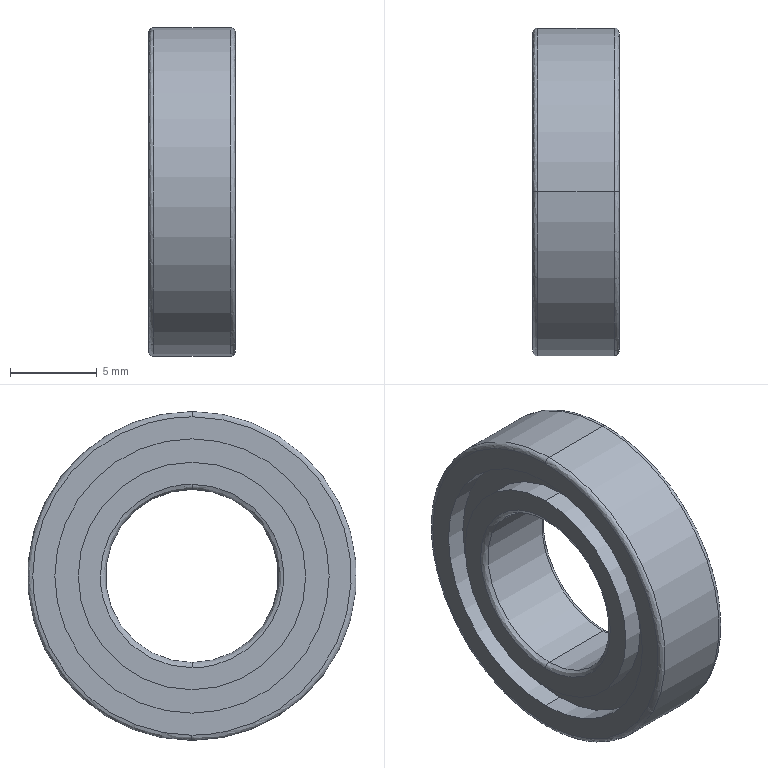Part | STEP file | B6800 | 1 solid | 26 faces | box 5 x 19 x 19 mm | volume 876.869 mm3 | cylinder 12 | spline 8 | plane 6 | commonest cylinder face diameters 13.15 x4 15.85 x4 10 x2 19 x2
STEP:
#1=CARTESIAN_POINT('',(0.,0.,9.2));
#2=VERTEX_POINT('',#1);
#3=CARTESIAN_POINT('',(0.,0.,-9.2));
#4=VERTEX_POINT('',#3);
#5=CARTESIAN_POINT('',(0.,0.,9.2));
#6=CARTESIAN_POINT('',(0.,-18.4,9.2));
#7=CARTESIAN_POINT('',(0.,-18.4,-9.2));
#8=CARTESIAN_POINT('',(0.,0.,-9.2));
#9=(BOUNDED_CURVE()B_SPLINE_CURVE(3,(#5,#6,#7,#8),.UNSPECIFIED.,.F.,.F.)B_SPLINE_CURVE_WITH_KNOTS((4,4),(0.,1.),.UNSPECIFIED.)CURVE()GEOMETRIC_REPRESENTATION_ITEM()RATIONAL_B_SPLINE_CURVE((1.,0.3333,0.3333,1.))REPRESENTATION_ITEM(''));
#10=EDGE_CURVE('',#2,#4,#9,.T.);
#11=ORIENTED_EDGE('',*,*,#10,.T.);
#12=CARTESIAN_POINT('',(0.3,0.,-9.5));
#13=VERTEX_POINT('',#12);
#14=CARTESIAN_POINT('',(0.3,0.,-9.2));
#15=DIRECTION('',(0.,-1.,0.));
#16=DIRECTION('',(0.,0.,-1.));
#17=AXIS2_PLACEMENT_3D('',#14,#15,#16);
#18=CIRCLE('',#17,0.3);
#19=EDGE_CURVE('',#4,#13,#18,.T.);
#20=ORIENTED_EDGE('',*,*,#19,.T.);
#21=CARTESIAN_POINT('',(0.3,0.,9.5));
#22=VERTEX_POINT('',#21);
#23=CARTESIAN_POINT('',(0.3,0.,0.));
#24=DIRECTION('',(1.,0.,0.));
#25=DIRECTION('',(0.,0.,-1.));
#26=AXIS2_PLACEMENT_3D('',#23,#24,#25);
#27=CIRCLE('',#26,9.5);
#28=EDGE_CURVE('',#22,#13,#27,.T.);
#29=ORIENTED_EDGE('',*,*,#28,.F.);
#30=CARTESIAN_POINT('',(0.3,0.,9.2));
#31=DIRECTION('',(0.,1.,0.));
#32=DIRECTION('',(0.,0.,1.));
#33=AXIS2_PLACEMENT_3D('',#30,#31,#32);
#34=CIRCLE('',#33,0.3);
#35=EDGE_CURVE('',#2,#22,#34,.T.);
#36=ORIENTED_EDGE('',*,*,#35,.F.);
#37=EDGE_LOOP('',(#11,#20,#29,#36));
#38=FACE_OUTER_BOUND('',#37,.T.);
#39=CARTESIAN_POINT('',(0.,0.,-9.2));
#40=CARTESIAN_POINT('',(0.,-18.4,-9.2));
#41=CARTESIAN_POINT('',(0.,-18.4,9.2));
#42=CARTESIAN_POINT('',(0.,0.,9.2));
#43=CARTESIAN_POINT('',(0.,0.,-9.376));
#44=CARTESIAN_POINT('',(0.,-18.751,-9.376));
#45=CARTESIAN_POINT('',(0.,-18.751,9.376));
#46=CARTESIAN_POINT('',(0.,0.,9.376));
#47=CARTESIAN_POINT('',(0.1243,0.,-9.5));
#48=CARTESIAN_POINT('',(0.1243,-19.,-9.5));
#49=CARTESIAN_POINT('',(0.1243,-19.,9.5));
#50=CARTESIAN_POINT('',(0.1243,0.,9.5));
#51=CARTESIAN_POINT('',(0.3,0.,-9.5));
#52=CARTESIAN_POINT('',(0.3,-19.,-9.5));
#53=CARTESIAN_POINT('',(0.3,-19.,9.5));
#54=CARTESIAN_POINT('',(0.3,0.,9.5));
#55=(BOUNDED_SURFACE()B_SPLINE_SURFACE(3,3,((#39,#40,#41,#42),(#43,#44,#45,#46),(#47,#48,#49,#50),(#51,#52,#53,#54)),.UNSPECIFIED.,.F.,.F.,.F.)B_SPLINE_SURFACE_WITH_KNOTS((4,4),(4,4),(0.,1.),(0.,1.),.UNSPECIFIED.)GEOMETRIC_REPRESENTATION_ITEM()RATIONAL_B_SPLINE_SURFACE(((1.,0.3333,0.3333,1.),(0.8047,0.2682,0.2682,0.8047),(0.8047,0.2682,0.2682,0.8047),(1.,0.3333,0.3333,1.)))REPRESENTATION_ITEM('')SURFACE());
#56=ADVANCED_FACE('',(#38),#55,.T.);
#57=CARTESIAN_POINT('',(4.7,0.,-9.5));
#58=VERTEX_POINT('',#57);
#59=CARTESIAN_POINT('',(4.7,0.,9.5));
#60=VERTEX_POINT('',#59);
#61=CARTESIAN_POINT('',(4.7,0.,0.));
#62=DIRECTION('',(-1.,0.,0.));
#63=DIRECTION('',(0.,0.,-1.));
#64=AXIS2_PLACEMENT_3D('',#61,#62,#63);
#65=CIRCLE('',#64,9.5);
#66=EDGE_CURVE('',#58,#60,#65,.T.);
#67=ORIENTED_EDGE('',*,*,#66,.F.);
#68=CARTESIAN_POINT('',(5.,0.,-9.2));
#69=VERTEX_POINT('',#68);
#70=CARTESIAN_POINT('',(4.7,0.,-9.2));
#71=DIRECTION('',(0.,-1.,0.));
#72=DIRECTION('',(0.,0.,-1.));
#73=AXIS2_PLACEMENT_3D('',#70,#71,#72);
#74=CIRCLE('',#73,0.3);
#75=EDGE_CURVE('',#58,#69,#74,.T.);
#76=ORIENTED_EDGE('',*,*,#75,.T.);
#77=CARTESIAN_POINT('',(5.,0.,9.2));
#78=VERTEX_POINT('',#77);
#79=CARTESIAN_POINT('',(5.,0.,-9.2));
#80=CARTESIAN_POINT('',(5.,-18.4,-9.2));
#81=CARTESIAN_POINT('',(5.,-18.4,9.2));
#82=CARTESIAN_POINT('',(5.,0.,9.2));
#83=(BOUNDED_CURVE()B_SPLINE_CURVE(3,(#79,#80,#81,#82),.UNSPECIFIED.,.F.,.F.)B_SPLINE_CURVE_WITH_KNOTS((4,4),(0.,1.),.UNSPECIFIED.)CURVE()GEOMETRIC_REPRESENTATION_ITEM()RATIONAL_B_SPLINE_CURVE((1.,0.3333,0.3333,1.))REPRESENTATION_ITEM(''));
#84=EDGE_CURVE('',#69,#78,#83,.T.);
#85=ORIENTED_EDGE('',*,*,#84,.T.);
#86=CARTESIAN_POINT('',(4.7,0.,9.2));
#87=DIRECTION('',(0.,1.,0.));
#88=DIRECTION('',(0.,0.,1.));
#89=AXIS2_PLACEMENT_3D('',#86,#87,#88);
#90=CIRCLE('',#89,0.3);
#91=EDGE_CURVE('',#60,#78,#90,.T.);
#92=ORIENTED_EDGE('',*,*,#91,.F.);
#93=EDGE_LOOP('',(#67,#76,#85,#92));
#94=FACE_OUTER_BOUND('',#93,.T.);
#95=CARTESIAN_POINT('',(4.7,0.,-9.5));
#96=CARTESIAN_POINT('',(4.7,-19.,-9.5));
#97=CARTESIAN_POINT('',(4.7,-19.,9.5));
#98=CARTESIAN_POINT('',(4.7,0.,9.5));
#99=CARTESIAN_POINT('',(4.876,0.,-9.5));
#100=CARTESIAN_POINT('',(4.876,-19.,-9.5));
#101=CARTESIAN_POINT('',(4.876,-19.,9.5));
#102=CARTESIAN_POINT('',(4.876,0.,9.5));
#103=CARTESIAN_POINT('',(5.,0.,-9.376));
#104=CARTESIAN_POINT('',(5.,-18.751,-9.376));
#105=CARTESIAN_POINT('',(5.,-18.751,9.376));
#106=CARTESIAN_POINT('',(5.,0.,9.376));
#107=CARTESIAN_POINT('',(5.,0.,-9.2));
#108=CARTESIAN_POINT('',(5.,-18.4,-9.2));
#109=CARTESIAN_POINT('',(5.,-18.4,9.2));
#110=CARTESIAN_POINT('',(5.,0.,9.2));
#111=(BOUNDED_SURFACE()B_SPLINE_SURFACE(3,3,((#95,#96,#97,#98),(#99,#100,#101,#102),(#103,#104,#105,#106),(#107,#108,#109,#110)),.UNSPECIFIED.,.F.,.F.,.F.)B_SPLINE_SURFACE_WITH_KNOTS((4,4),(4,4),(0.,1.),(0.,1.),.UNSPECIFIED.)GEOMETRIC_REPRESENTATION_ITEM()RATIONAL_B_SPLINE_SURFACE(((1.,0.3333,0.3333,1.),(0.8047,0.2682,0.2682,0.8047),(0.8047,0.2682,0.2682,0.8047),(1.,0.3333,0.3333,1.)))REPRESENTATION_ITEM('')SURFACE());
#112=ADVANCED_FACE('',(#94),#111,.T.);
#113=CARTESIAN_POINT('',(0.3,0.,5.));
#114=VERTEX_POINT('',#113);
#115=CARTESIAN_POINT('',(0.3,0.,-5.));
#116=VERTEX_POINT('',#115);
#117=CARTESIAN_POINT('',(0.3,0.,0.));
#118=DIRECTION('',(1.,0.,0.));
#119=DIRECTION('',(0.,0.,1.));
#120=AXIS2_PLACEMENT_3D('',#117,#118,#119);
#121=CIRCLE('',#120,5.);
#122=EDGE_CURVE('',#114,#116,#121,.T.);
#123=ORIENTED_EDGE('',*,*,#122,.T.);
#124=CARTESIAN_POINT('',(0.,0.,-5.3));
#125=VERTEX_POINT('',#124);
#126=CARTESIAN_POINT('',(0.3,0.,-5.3));
#127=DIRECTION('',(0.,-1.,0.));
#128=DIRECTION('',(0.,0.,-1.));
#129=AXIS2_PLACEMENT_3D('',#126,#127,#128);
#130=CIRCLE('',#129,0.3);
#131=EDGE_CURVE('',#116,#125,#130,.T.);
#132=ORIENTED_EDGE('',*,*,#131,.T.);
#133=CARTESIAN_POINT('',(0.,0.,5.3));
#134=VERTEX_POINT('',#133);
#135=CARTESIAN_POINT('',(0.,0.,5.3));
#136=CARTESIAN_POINT('',(0.,-0.3371,5.3));
#137=CARTESIAN_POINT('',(0.,-0.8337,5.253));
#138=CARTESIAN_POINT('',(0.,-1.398,5.118));
#139=CARTESIAN_POINT('',(0.,-1.676,5.03));
#140=CARTESIAN_POINT('',(0.,-1.814,4.98));
#141=CARTESIAN_POINT('',(0.,-1.872,4.958));
#142=CARTESIAN_POINT('',(0.,-1.912,4.943));
#143=CARTESIAN_POINT('',(0.,-1.93,4.936));
#144=CARTESIAN_POINT('',(0.,-2.117,4.862));
#145=CARTESIAN_POINT('',(0.,-2.361,4.751));
#146=CARTESIAN_POINT('',(0.,-2.595,4.622));
#147=CARTESIAN_POINT('',(0.,-2.749,4.532));
#148=CARTESIAN_POINT('',(0.,-2.824,4.486));
#149=CARTESIAN_POINT('',(0.,-3.206,4.236));
#150=CARTESIAN_POINT('',(0.,-3.489,4.006));
#151=CARTESIAN_POINT('',(0.,-3.877,3.618));
#152=CARTESIAN_POINT('',(0.,-4.06,3.416));
#153=CARTESIAN_POINT('',(0.,-4.227,3.199));
#154=CARTESIAN_POINT('',(0.,-4.334,3.052));
#155=CARTESIAN_POINT('',(0.,-4.387,2.975));
#156=CARTESIAN_POINT('',(0.,-4.534,2.75));
#157=CARTESIAN_POINT('',(0.,-4.669,2.519));
#158=CARTESIAN_POINT('',(0.,-4.805,2.239));
#159=CARTESIAN_POINT('',(0.,-4.859,2.116));
#160=CARTESIAN_POINT('',(0.,-4.894,2.034));
#161=CARTESIAN_POINT('',(0.,-4.912,1.991));
#162=CARTESIAN_POINT('',(0.,-4.991,1.791));
#163=CARTESIAN_POINT('',(0.,-5.074,1.548));
#164=CARTESIAN_POINT('',(0.,-5.15,1.258));
#165=CARTESIAN_POINT('',(0.,-5.182,1.112));
#166=CARTESIAN_POINT('',(0.,-5.195,1.049));
#167=CARTESIAN_POINT('',(0.,-5.204,1.007));
#168=CARTESIAN_POINT('',(0.,-5.208,0.9843));
#169=CARTESIAN_POINT('',(0.,-5.27,0.646));
#170=CARTESIAN_POINT('',(0.,-5.3,0.3238));
#171=CARTESIAN_POINT('',(0.,-5.3,-0.1619));
#172=CARTESIAN_POINT('',(0.,-5.289,-0.4039));
#173=CARTESIAN_POINT('',(0.,-5.257,-0.6847));
#174=CARTESIAN_POINT('',(0.,-5.236,-0.8247));
#175=CARTESIAN_POINT('',(0.,-5.226,-0.8846));
#176=CARTESIAN_POINT('',(0.,-5.219,-0.9245));
#177=CARTESIAN_POINT('',(0.,-5.215,-0.9433));
#178=CARTESIAN_POINT('',(0.,-5.18,-1.133));
#179=CARTESIAN_POINT('',(0.,-5.121,-1.383));
#180=CARTESIAN_POINT('',(0.,-5.032,-1.669));
#181=CARTESIAN_POINT('',(0.,-4.989,-1.79));
#182=CARTESIAN_POINT('',(0.,-4.959,-1.871));
#183=CARTESIAN_POINT('',(0.,-4.944,-1.909));
#184=CARTESIAN_POINT('',(0.,-4.862,-2.117));
#185=CARTESIAN_POINT('',(0.,-4.751,-2.361));
#186=CARTESIAN_POINT('',(0.,-4.622,-2.595));
#187=CARTESIAN_POINT('',(0.,-4.532,-2.749));
#188=CARTESIAN_POINT('',(0.,-4.486,-2.824));
#189=CARTESIAN_POINT('',(0.,-4.236,-3.206));
#190=CARTESIAN_POINT('',(0.,-4.006,-3.489));
#191=CARTESIAN_POINT('',(0.,-3.618,-3.877));
#192=CARTESIAN_POINT('',(0.,-3.416,-4.06));
#193=CARTESIAN_POINT('',(0.,-3.199,-4.227));
#194=CARTESIAN_POINT('',(0.,-3.052,-4.334));
#195=CARTESIAN_POINT('',(0.,-2.975,-4.387));
#196=CARTESIAN_POINT('',(0.,-2.75,-4.534));
#197=CARTESIAN_POINT('',(0.,-2.519,-4.669));
#198=CARTESIAN_POINT('',(0.,-2.239,-4.805));
#199=CARTESIAN_POINT('',(0.,-2.116,-4.859));
#200=CARTESIAN_POINT('',(0.,-2.034,-4.894));
#201=CARTESIAN_POINT('',(0.,-1.991,-4.912));
#202=CARTESIAN_POINT('',(0.,-1.791,-4.991));
#203=CARTESIAN_POINT('',(0.,-1.548,-5.074));
#204=CARTESIAN_POINT('',(0.,-1.258,-5.15));
#205=CARTESIAN_POINT('',(0.,-1.112,-5.182));
#206=CARTESIAN_POINT('',(0.,-1.049,-5.195));
#207=CARTESIAN_POINT('',(0.,-1.007,-5.204));
#208=CARTESIAN_POINT('',(0.,-0.9843,-5.208));
#209=CARTESIAN_POINT('',(0.,-0.6462,-5.27));
#210=CARTESIAN_POINT('',(0.,-0.3247,-5.3));
#211=CARTESIAN_POINT('',(0.,0.,-5.3));
#212=B_SPLINE_CURVE_WITH_KNOTS('',3,(#135,#136,#137,#138,#139,#140,#141,#142,#143,#144,#145,#146,#147,#148,#149,#150,#151,#152,#153,#154,#155,#156,#157,#158,#159,#160,#161,#162,#163,#164,#165,#166,#167,#168,#169,#170,#171,#172,#173,#174,#175,#176,#177,#178,#179,#180,#181,#182,#183,#184,#185,#186,#187,#188,#189,#190,#191,#192,#193,#194,#195,#196,#197,#198,#199,#200,#201,#202,#203,#204,#205,#206,#207,#208,#209,#210,#211),.UNSPECIFIED.,.F.,.F.,(4,1,1,1,1,2,2,1,2,2,2,1,2,2,1,1,2,2,1,1,1,2,2,2,1,1,1,2,2,1,1,2,2,1,2,2,2,1,2,2,1,1,2,2,1,1,1,2,2,4),(0.,0.0625,0.09375,0.1094,0.1172,0.1211,0.125,0.1563,0.1719,0.1875,0.25,0.2813,0.2969,0.3125,0.3438,0.3594,0.3672,0.375,0.4062,0.4219,0.4297,0.4336,0.4375,0.5,0.5312,0.5469,0.5547,0.5586,0.5625,0.5937,0.6094,0.6172,0.625,0.6562,0.6719,0.6875,0.75,0.7812,0.7969,0.8125,0.8437,0.8594,0.8672,0.875,0.9062,0.9219,0.9297,0.9336,0.9375,1.),.UNSPECIFIED.);
#213=EDGE_CURVE('',#134,#125,#212,.T.);
#214=ORIENTED_EDGE('',*,*,#213,.F.);
#215=CARTESIAN_POINT('',(0.3,0.,5.3));
#216=DIRECTION('',(0.,1.,0.));
#217=DIRECTION('',(0.,0.,1.));
#218=AXIS2_PLACEMENT_3D('',#215,#216,#217);
#219=CIRCLE('',#218,0.3);
#220=EDGE_CURVE('',#114,#134,#219,.T.);
#221=ORIENTED_EDGE('',*,*,#220,.F.);
#222=EDGE_LOOP('',(#123,#132,#214,#221));
#223=FACE_OUTER_BOUND('',#222,.T.);
#224=CARTESIAN_POINT('',(0.3,0.,-5.));
#225=CARTESIAN_POINT('',(0.3,-10.,-5.));
#226=CARTESIAN_POINT('',(0.3,-10.,5.));
#227=CARTESIAN_POINT('',(0.3,0.,5.));
#228=CARTESIAN_POINT('',(0.1243,0.,-5.));
#229=CARTESIAN_POINT('',(0.1243,-10.,-5.));
#230=CARTESIAN_POINT('',(0.1243,-10.,5.));
#231=CARTESIAN_POINT('',(0.1243,0.,5.));
#232=CARTESIAN_POINT('',(0.,0.,-5.124));
#233=CARTESIAN_POINT('',(0.,-10.249,-5.124));
#234=CARTESIAN_POINT('',(0.,-10.249,5.124));
#235=CARTESIAN_POINT('',(0.,0.,5.124));
#236=CARTESIAN_POINT('',(0.,0.,-5.3));
#237=CARTESIAN_POINT('',(0.,-10.6,-5.3));
#238=CARTESIAN_POINT('',(0.,-10.6,5.3));
#239=CARTESIAN_POINT('',(0.,0.,5.3));
#240=(BOUNDED_SURFACE()B_SPLINE_SURFACE(3,3,((#224,#225,#226,#227),(#228,#229,#230,#231),(#232,#233,#234,#235),(#236,#237,#238,#239)),.UNSPECIFIED.,.F.,.F.,.F.)B_SPLINE_SURFACE_WITH_KNOTS((4,4),(4,4),(0.,1.),(0.,1.),.UNSPECIFIED.)GEOMETRIC_REPRESENTATION_ITEM()RATIONAL_B_SPLINE_SURFACE(((1.,0.3333,0.3333,1.),(0.8047,0.2682,0.2682,0.8047),(0.8047,0.2682,0.2682,0.8047),(1.,0.3333,0.3333,1.)))REPRESENTATION_ITEM('')SURFACE());
#241=ADVANCED_FACE('',(#223),#240,.T.);
#242=CARTESIAN_POINT('',(5.,0.,-5.3));
#243=VERTEX_POINT('',#242);
#244=CARTESIAN_POINT('',(5.,0.,5.3));
#245=VERTEX_POINT('',#244);
#246=CARTESIAN_POINT('',(5.,0.,-5.3));
#247=CARTESIAN_POINT('',(5.,-0.3371,-5.3));
#248=CARTESIAN_POINT('',(5.,-0.8337,-5.253));
#249=CARTESIAN_POINT('',(5.,-1.398,-5.118));
#250=CARTESIAN_POINT('',(5.,-1.676,-5.03));
#251=CARTESIAN_POINT('',(5.,-1.814,-4.98));
#252=CARTESIAN_POINT('',(5.,-1.872,-4.958));
#253=CARTESIAN_POINT('',(5.,-1.912,-4.943));
#254=CARTESIAN_POINT('',(5.,-1.93,-4.936));
#255=CARTESIAN_POINT('',(5.,-2.117,-4.862));
#256=CARTESIAN_POINT('',(5.,-2.361,-4.751));
#257=CARTESIAN_POINT('',(5.,-2.595,-4.622));
#258=CARTESIAN_POINT('',(5.,-2.749,-4.532));
#259=CARTESIAN_POINT('',(5.,-2.824,-4.486));
#260=CARTESIAN_POINT('',(5.,-3.206,-4.236));
#261=CARTESIAN_POINT('',(5.,-3.489,-4.006));
#262=CARTESIAN_POINT('',(5.,-3.877,-3.618));
#263=CARTESIAN_POINT('',(5.,-4.06,-3.416));
#264=CARTESIAN_POINT('',(5.,-4.227,-3.199));
#265=CARTESIAN_POINT('',(5.,-4.334,-3.052));
#266=CARTESIAN_POINT('',(5.,-4.387,-2.975));
#267=CARTESIAN_POINT('',(5.,-4.534,-2.75));
#268=CARTESIAN_POINT('',(5.,-4.669,-2.519));
#269=CARTESIAN_POINT('',(5.,-4.805,-2.239));
#270=CARTESIAN_POINT('',(5.,-4.859,-2.116));
#271=CARTESIAN_POINT('',(5.,-4.894,-2.034));
#272=CARTESIAN_POINT('',(5.,-4.912,-1.991));
#273=CARTESIAN_POINT('',(5.,-4.991,-1.791));
#274=CARTESIAN_POINT('',(5.,-5.074,-1.548));
#275=CARTESIAN_POINT('',(5.,-5.15,-1.258));
#276=CARTESIAN_POINT('',(5.,-5.182,-1.112));
#277=CARTESIAN_POINT('',(5.,-5.195,-1.049));
#278=CARTESIAN_POINT('',(5.,-5.204,-1.007));
#279=CARTESIAN_POINT('',(5.,-5.208,-0.9843));
#280=CARTESIAN_POINT('',(5.,-5.27,-0.646));
#281=CARTESIAN_POINT('',(5.,-5.3,-0.3238));
#282=CARTESIAN_POINT('',(5.,-5.3,0.1619));
#283=CARTESIAN_POINT('',(5.,-5.289,0.4039));
#284=CARTESIAN_POINT('',(5.,-5.257,0.6847));
#285=CARTESIAN_POINT('',(5.,-5.236,0.8247));
#286=CARTESIAN_POINT('',(5.,-5.226,0.8846));
#287=CARTESIAN_POINT('',(5.,-5.219,0.9245));
#288=CARTESIAN_POINT('',(5.,-5.215,0.9433));
#289=CARTESIAN_POINT('',(5.,-5.18,1.133));
#290=CARTESIAN_POINT('',(5.,-5.121,1.383));
#291=CARTESIAN_POINT('',(5.,-5.032,1.669));
#292=CARTESIAN_POINT('',(5.,-4.989,1.79));
#293=CARTESIAN_POINT('',(5.,-4.959,1.871));
#294=CARTESIAN_POINT('',(5.,-4.944,1.909));
#295=CARTESIAN_POINT('',(5.,-4.862,2.117));
#296=CARTESIAN_POINT('',(5.,-4.751,2.361));
#297=CARTESIAN_POINT('',(5.,-4.622,2.595));
#298=CARTESIAN_POINT('',(5.,-4.532,2.749));
#299=CARTESIAN_POINT('',(5.,-4.486,2.824));
#300=CARTESIAN_POINT('',(5.,-4.236,3.206));
#301=CARTESIAN_POINT('',(5.,-4.006,3.489));
#302=CARTESIAN_POINT('',(5.,-3.618,3.877));
#303=CARTESIAN_POINT('',(5.,-3.416,4.06));
#304=CARTESIAN_POINT('',(5.,-3.199,4.227));
#305=CARTESIAN_POINT('',(5.,-3.052,4.334));
#306=CARTESIAN_POINT('',(5.,-2.975,4.387));
#307=CARTESIAN_POINT('',(5.,-2.75,4.534));
#308=CARTESIAN_POINT('',(5.,-2.519,4.669));
#309=CARTESIAN_POINT('',(5.,-2.239,4.805));
#310=CARTESIAN_POINT('',(5.,-2.116,4.859));
#311=CARTESIAN_POINT('',(5.,-2.034,4.894));
#312=CARTESIAN_POINT('',(5.,-1.991,4.912));
#313=CARTESIAN_POINT('',(5.,-1.791,4.991));
#314=CARTESIAN_POINT('',(5.,-1.548,5.074));
#315=CARTESIAN_POINT('',(5.,-1.258,5.15));
#316=CARTESIAN_POINT('',(5.,-1.112,5.182));
#317=CARTESIAN_POINT('',(5.,-1.049,5.195));
#318=CARTESIAN_POINT('',(5.,-1.007,5.204));
#319=CARTESIAN_POINT('',(5.,-0.9843,5.208));
#320=CARTESIAN_POINT('',(5.,-0.6462,5.27));
#321=CARTESIAN_POINT('',(5.,-0.3247,5.3));
#322=CARTESIAN_POINT('',(5.,0.,5.3));
#323=B_SPLINE_CURVE_WITH_KNOTS('',3,(#246,#247,#248,#249,#250,#251,#252,#253,#254,#255,#256,#257,#258,#259,#260,#261,#262,#263,#264,#265,#266,#267,#268,#269,#270,#271,#272,#273,#274,#275,#276,#277,#278,#279,#280,#281,#282,#283,#284,#285,#286,#287,#288,#289,#290,#291,#292,#293,#294,#295,#296,#297,#298,#299,#300,#301,#302,#303,#304,#305,#306,#307,#308,#309,#310,#311,#312,#313,#314,#315,#316,#317,#318,#319,#320,#321,#322),.UNSPECIFIED.,.F.,.F.,(4,1,1,1,1,2,2,1,2,2,2,1,2,2,1,1,2,2,1,1,1,2,2,2,1,1,1,2,2,1,1,2,2,1,2,2,2,1,2,2,1,1,2,2,1,1,1,2,2,4),(0.,0.0625,0.09375,0.1094,0.1172,0.1211,0.125,0.1563,0.1719,0.1875,0.25,0.2813,0.2969,0.3125,0.3438,0.3594,0.3672,0.375,0.4063,0.4219,0.4297,0.4336,0.4375,0.5,0.5312,0.5469,0.5547,0.5586,0.5625,0.5937,0.6094,0.6172,0.625,0.6562,0.6719,0.6875,0.75,0.7812,0.7969,0.8125,0.8437,0.8594,0.8672,0.875,0.9062,0.9219,0.9297,0.9336,0.9375,1.),.UNSPECIFIED.);
#324=EDGE_CURVE('',#243,#245,#323,.T.);
#325=ORIENTED_EDGE('',*,*,#324,.F.);
#326=CARTESIAN_POINT('',(4.7,0.,-5.));
#327=VERTEX_POINT('',#326);
#328=CARTESIAN_POINT('',(4.7,0.,-5.3));
#329=DIRECTION('',(0.,-1.,0.));
#330=DIRECTION('',(0.,0.,-1.));
#331=AXIS2_PLACEMENT_3D('',#328,#329,#330);
#332=CIRCLE('',#331,0.3);
#333=EDGE_CURVE('',#243,#327,#332,.T.);
#334=ORIENTED_EDGE('',*,*,#333,.T.);
#335=CARTESIAN_POINT('',(4.7,0.,5.));
#336=VERTEX_POINT('',#335);
#337=CARTESIAN_POINT('',(4.7,0.,0.));
#338=DIRECTION('',(-1.,0.,0.));
#339=DIRECTION('',(0.,0.,1.));
#340=AXIS2_PLACEMENT_3D('',#337,#338,#339);
#341=CIRCLE('',#340,5.);
#342=EDGE_CURVE('',#327,#336,#341,.T.);
#343=ORIENTED_EDGE('',*,*,#342,.T.);
#344=CARTESIAN_POINT('',(4.7,0.,5.3));
#345=DIRECTION('',(0.,1.,0.));
#346=DIRECTION('',(0.,0.,1.));
#347=AXIS2_PLACEMENT_3D('',#344,#345,#346);
#348=CIRCLE('',#347,0.3);
#349=EDGE_CURVE('',#245,#336,#348,.T.);
#350=ORIENTED_EDGE('',*,*,#349,.F.);
#351=EDGE_LOOP('',(#325,#334,#343,#350));
#352=FACE_OUTER_BOUND('',#351,.T.);
#353=CARTESIAN_POINT('',(5.,0.,-5.3));
#354=CARTESIAN_POINT('',(5.,-10.6,-5.3));
#355=CARTESIAN_POINT('',(5.,-10.6,5.3));
#356=CARTESIAN_POINT('',(5.,0.,5.3));
#357=CARTESIAN_POINT('',(5.,0.,-5.124));
#358=CARTESIAN_POINT('',(5.,-10.249,-5.124));
#359=CARTESIAN_POINT('',(5.,-10.249,5.124));
#360=CARTESIAN_POINT('',(5.,0.,5.124));
#361=CARTESIAN_POINT('',(4.876,0.,-5.));
#362=CARTESIAN_POINT('',(4.876,-10.,-5.));
#363=CARTESIAN_POINT('',(4.876,-10.,5.));
#364=CARTESIAN_POINT('',(4.876,0.,5.));
#365=CARTESIAN_POINT('',(4.7,0.,-5.));
#366=CARTESIAN_POINT('',(4.7,-10.,-5.));
#367=CARTESIAN_POINT('',(4.7,-10.,5.));
#368=CARTESIAN_POINT('',(4.7,0.,5.));
#369=(BOUNDED_SURFACE()B_SPLINE_SURFACE(3,3,((#353,#354,#355,#356),(#357,#358,#359,#360),(#361,#362,#363,#364),(#365,#366,#367,#368)),.UNSPECIFIED.,.F.,.F.,.F.)B_SPLINE_SURFACE_WITH_KNOTS((4,4),(4,4),(0.,1.),(0.,1.),.UNSPECIFIED.)GEOMETRIC_REPRESENTATION_ITEM()RATIONAL_B_SPLINE_SURFACE(((1.,0.3333,0.3333,1.),(0.8047,0.2682,0.2682,0.8047),(0.8047,0.2682,0.2682,0.8047),(1.,0.3333,0.3333,1.)))REPRESENTATION_ITEM('')SURFACE());
#370=ADVANCED_FACE('',(#352),#369,.T.);
#371=CARTESIAN_POINT('',(0.3,0.,0.));
#372=DIRECTION('',(1.,0.,0.));
#373=DIRECTION('',(0.,0.,-1.));
#374=AXIS2_PLACEMENT_3D('',#371,#372,#373);
#375=CIRCLE('',#374,9.5);
#376=EDGE_CURVE('',#13,#22,#375,.T.);
#377=ORIENTED_EDGE('',*,*,#376,.T.);
#378=CARTESIAN_POINT('',(2.5,0.,9.5));
#379=DIRECTION('',(1.,0.,0.));
#380=VECTOR('',#379,1000.);
#381=LINE('',#378,#380);
#382=EDGE_CURVE('',#22,#60,#381,.T.);
#383=ORIENTED_EDGE('',*,*,#382,.T.);
#384=CARTESIAN_POINT('',(4.7,0.,0.));
#385=DIRECTION('',(-1.,0.,0.));
#386=DIRECTION('',(0.,0.,-1.));
#387=AXIS2_PLACEMENT_3D('',#384,#385,#386);
#388=CIRCLE('',#387,9.5);
#389=EDGE_CURVE('',#60,#58,#388,.T.);
#390=ORIENTED_EDGE('',*,*,#389,.T.);
#391=CARTESIAN_POINT('',(2.5,0.,-9.5));
#392=DIRECTION('',(1.,0.,0.));
#393=VECTOR('',#392,1000.);
#394=LINE('',#391,#393);
#395=EDGE_CURVE('',#13,#58,#394,.T.);
#396=ORIENTED_EDGE('',*,*,#395,.F.);
#397=EDGE_LOOP('',(#377,#383,#390,#396));
#398=FACE_OUTER_BOUND('',#397,.T.);
#399=CARTESIAN_POINT('',(2.5,0.,0.));
#400=DIRECTION('',(1.,0.,0.));
#401=DIRECTION('',(0.,0.,-1.));
#402=AXIS2_PLACEMENT_3D('',#399,#400,#401);
#403=CYLINDRICAL_SURFACE('',#402,9.5);
#404=ADVANCED_FACE('',(#398),#403,.T.);
#405=CARTESIAN_POINT('',(0.,0.,7.925));
#406=VERTEX_POINT('',#405);
#407=CARTESIAN_POINT('',(0.,0.,-7.925));
#408=VERTEX_POINT('',#407);
#409=CARTESIAN_POINT('',(0.,0.,0.));
#410=DIRECTION('',(1.,0.,0.));
#411=DIRECTION('',(0.,0.,-1.));
#412=AXIS2_PLACEMENT_3D('',#409,#410,#411);
#413=CIRCLE('',#412,7.925);
#414=EDGE_CURVE('',#406,#408,#413,.T.);
#415=ORIENTED_EDGE('',*,*,#414,.F.);
#416=CARTESIAN_POINT('',(1.175,0.,7.925));
#417=VERTEX_POINT('',#416);
#418=CARTESIAN_POINT('',(0.5875,0.,7.925));
#419=DIRECTION('',(1.,0.,0.));
#420=VECTOR('',#419,1000.);
#421=LINE('',#418,#420);
#422=EDGE_CURVE('',#406,#417,#421,.T.);
#423=ORIENTED_EDGE('',*,*,#422,.T.);
#424=CARTESIAN_POINT('',(1.175,0.,-7.925));
#425=VERTEX_POINT('',#424);
#426=CARTESIAN_POINT('',(1.175,0.,0.));
#427=DIRECTION('',(-1.,0.,0.));
#428=DIRECTION('',(0.,0.,-1.));
#429=AXIS2_PLACEMENT_3D('',#426,#427,#428);
#430=CIRCLE('',#429,7.925);
#431=EDGE_CURVE('',#425,#417,#430,.T.);
#432=ORIENTED_EDGE('',*,*,#431,.F.);
#433=CARTESIAN_POINT('',(0.5875,0.,-7.925));
#434=DIRECTION('',(1.,0.,0.));
#435=VECTOR('',#434,1000.);
#436=LINE('',#433,#435);
#437=EDGE_CURVE('',#408,#425,#436,.T.);
#438=ORIENTED_EDGE('',*,*,#437,.F.);
#439=EDGE_LOOP('',(#415,#423,#432,#438));
#440=FACE_OUTER_BOUND('',#439,.T.);
#441=CARTESIAN_POINT('',(0.5875,0.,0.));
#442=DIRECTION('',(1.,0.,0.));
#443=DIRECTION('',(0.,0.,-1.));
#444=AXIS2_PLACEMENT_3D('',#441,#442,#443);
#445=CYLINDRICAL_SURFACE('',#444,7.925);
#446=ADVANCED_FACE('',(#440),#445,.F.);
#447=CARTESIAN_POINT('',(3.825,0.,7.925));
#448=VERTEX_POINT('',#447);
#449=CARTESIAN_POINT('',(3.825,0.,-7.925));
#450=VERTEX_POINT('',#449);
#451=CARTESIAN_POINT('',(3.825,0.,0.));
#452=DIRECTION('',(1.,0.,0.));
#453=DIRECTION('',(0.,0.,-1.));
#454=AXIS2_PLACEMENT_3D('',#451,#452,#453);
#455=CIRCLE('',#454,7.925);
#456=EDGE_CURVE('',#448,#450,#455,.T.);
#457=ORIENTED_EDGE('',*,*,#456,.F.);
#458=CARTESIAN_POINT('',(5.,0.,7.925));
#459=VERTEX_POINT('',#458);
#460=CARTESIAN_POINT('',(4.412,0.,7.925));
#461=DIRECTION('',(1.,0.,0.));
#462=VECTOR('',#461,1000.);
#463=LINE('',#460,#462);
#464=EDGE_CURVE('',#448,#459,#463,.T.);
#465=ORIENTED_EDGE('',*,*,#464,.T.);
#466=CARTESIAN_POINT('',(5.,0.,-7.925));
#467=VERTEX_POINT('',#466);
#468=CARTESIAN_POINT('',(5.,0.,0.));
#469=DIRECTION('',(-1.,0.,0.));
#470=DIRECTION('',(0.,0.,-1.));
#471=AXIS2_PLACEMENT_3D('',#468,#469,#470);
#472=CIRCLE('',#471,7.925);
#473=EDGE_CURVE('',#467,#459,#472,.T.);
#474=ORIENTED_EDGE('',*,*,#473,.F.);
#475=CARTESIAN_POINT('',(4.412,0.,-7.925));
#476=DIRECTION('',(1.,0.,0.));
#477=VECTOR('',#476,1000.);
#478=LINE('',#475,#477);
#479=EDGE_CURVE('',#450,#467,#478,.T.);
#480=ORIENTED_EDGE('',*,*,#479,.F.);
#481=EDGE_LOOP('',(#457,#465,#474,#480));
#482=FACE_OUTER_BOUND('',#481,.T.);
#483=CARTESIAN_POINT('',(4.412,0.,0.));
#484=DIRECTION('',(1.,0.,0.));
#485=DIRECTION('',(0.,0.,-1.));
#486=AXIS2_PLACEMENT_3D('',#483,#484,#485);
#487=CYLINDRICAL_SURFACE('',#486,7.925);
#488=ADVANCED_FACE('',(#482),#487,.F.);
#489=CARTESIAN_POINT('',(0.,0.,-6.575));
#490=VERTEX_POINT('',#489);
#491=CARTESIAN_POINT('',(0.,0.,6.575));
#492=VERTEX_POINT('',#491);
#493=CARTESIAN_POINT('',(0.,0.,0.));
#494=DIRECTION('',(1.,0.,0.));
#495=DIRECTION('',(0.,0.,-1.));
#496=AXIS2_PLACEMENT_3D('',#493,#494,#495);
#497=CIRCLE('',#496,6.575);
#498=EDGE_CURVE('',#490,#492,#497,.T.);
#499=ORIENTED_EDGE('',*,*,#498,.T.);
#500=CARTESIAN_POINT('',(1.175,0.,6.575));
#501=VERTEX_POINT('',#500);
#502=CARTESIAN_POINT('',(0.5875,0.,6.575));
#503=DIRECTION('',(1.,0.,0.));
#504=VECTOR('',#503,1000.);
#505=LINE('',#502,#504);
#506=EDGE_CURVE('',#492,#501,#505,.T.);
#507=ORIENTED_EDGE('',*,*,#506,.T.);
#508=CARTESIAN_POINT('',(1.175,0.,-6.575));
#509=VERTEX_POINT('',#508);
#510=CARTESIAN_POINT('',(1.175,0.,0.));
#511=DIRECTION('',(1.,0.,0.));
#512=DIRECTION('',(0.,0.,-1.));
#513=AXIS2_PLACEMENT_3D('',#510,#511,#512);
#514=CIRCLE('',#513,6.575);
#515=EDGE_CURVE('',#509,#501,#514,.T.);
#516=ORIENTED_EDGE('',*,*,#515,.F.);
#517=CARTESIAN_POINT('',(0.5875,0.,-6.575));
#518=DIRECTION('',(1.,0.,0.));
#519=VECTOR('',#518,1000.);
#520=LINE('',#517,#519);
#521=EDGE_CURVE('',#490,#509,#520,.T.);
#522=ORIENTED_EDGE('',*,*,#521,.F.);
#523=EDGE_LOOP('',(#499,#507,#516,#522));
#524=FACE_OUTER_BOUND('',#523,.T.);
#525=CARTESIAN_POINT('',(0.5875,0.,0.));
#526=DIRECTION('',(1.,0.,0.));
#527=DIRECTION('',(0.,0.,-1.));
#528=AXIS2_PLACEMENT_3D('',#525,#526,#527);
#529=CYLINDRICAL_SURFACE('',#528,6.575);
#530=ADVANCED_FACE('',(#524),#529,.T.);
#531=CARTESIAN_POINT('',(3.825,0.,6.575));
#532=VERTEX_POINT('',#531);
#533=CARTESIAN_POINT('',(3.825,0.,-6.575));
#534=VERTEX_POINT('',#533);
#535=CARTESIAN_POINT('',(3.825,0.,0.));
#536=DIRECTION('',(-1.,0.,0.));
#537=DIRECTION('',(0.,0.,-1.));
#538=AXIS2_PLACEMENT_3D('',#535,#536,#537);
#539=CIRCLE('',#538,6.575);
#540=EDGE_CURVE('',#532,#534,#539,.T.);
#541=ORIENTED_EDGE('',*,*,#540,.F.);
#542=CARTESIAN_POINT('',(5.,0.,6.575));
#543=VERTEX_POINT('',#542);
#544=CARTESIAN_POINT('',(4.412,0.,6.575));
#545=DIRECTION('',(1.,0.,0.));
#546=VECTOR('',#545,1000.);
#547=LINE('',#544,#546);
#548=EDGE_CURVE('',#532,#543,#547,.T.);
#549=ORIENTED_EDGE('',*,*,#548,.T.);
#550=CARTESIAN_POINT('',(5.,0.,-6.575));
#551=VERTEX_POINT('',#550);
#552=CARTESIAN_POINT('',(5.,0.,0.));
#553=DIRECTION('',(-1.,0.,0.));
#554=DIRECTION('',(0.,0.,-1.));
#555=AXIS2_PLACEMENT_3D('',#552,#553,#554);
#556=CIRCLE('',#555,6.575);
#557=EDGE_CURVE('',#543,#551,#556,.T.);
#558=ORIENTED_EDGE('',*,*,#557,.T.);
#559=CARTESIAN_POINT('',(4.412,0.,-6.575));
#560=DIRECTION('',(1.,0.,0.));
#561=VECTOR('',#560,1000.);
#562=LINE('',#559,#561);
#563=EDGE_CURVE('',#534,#551,#562,.T.);
#564=ORIENTED_EDGE('',*,*,#563,.F.);
#565=EDGE_LOOP('',(#541,#549,#558,#564));
#566=FACE_OUTER_BOUND('',#565,.T.);
#567=CARTESIAN_POINT('',(4.412,0.,0.));
#568=DIRECTION('',(1.,0.,0.));
#569=DIRECTION('',(0.,0.,-1.));
#570=AXIS2_PLACEMENT_3D('',#567,#568,#569);
#571=CYLINDRICAL_SURFACE('',#570,6.575);
#572=ADVANCED_FACE('',(#566),#571,.T.);
#573=ORIENTED_EDGE('',*,*,#122,.F.);
#574=CARTESIAN_POINT('',(2.5,0.,5.));
#575=DIRECTION('',(1.,0.,0.));
#576=VECTOR('',#575,1000.);
#577=LINE('',#574,#576);
#578=EDGE_CURVE('',#114,#336,#577,.T.);
#579=ORIENTED_EDGE('',*,*,#578,.T.);
#580=ORIENTED_EDGE('',*,*,#342,.F.);
#581=CARTESIAN_POINT('',(2.5,0.,-5.));
#582=DIRECTION('',(1.,0.,0.));
#583=VECTOR('',#582,1000.);
#584=LINE('',#581,#583);
#585=EDGE_CURVE('',#116,#327,#584,.T.);
#586=ORIENTED_EDGE('',*,*,#585,.F.);
#587=EDGE_LOOP('',(#573,#579,#580,#586));
#588=FACE_OUTER_BOUND('',#587,.T.);
#589=CARTESIAN_POINT('',(2.5,0.,0.));
#590=DIRECTION('',(1.,0.,0.));
#591=DIRECTION('',(0.,0.,-1.));
#592=AXIS2_PLACEMENT_3D('',#589,#590,#591);
#593=CYLINDRICAL_SURFACE('',#592,5.);
#594=ADVANCED_FACE('',(#588),#593,.F.);
#595=ORIENTED_EDGE('',*,*,#382,.F.);
#596=ORIENTED_EDGE('',*,*,#28,.T.);
#597=ORIENTED_EDGE('',*,*,#395,.T.);
#598=ORIENTED_EDGE('',*,*,#66,.T.);
#599=EDGE_LOOP('',(#595,#596,#597,#598));
#600=FACE_OUTER_BOUND('',#599,.T.);
#601=CARTESIAN_POINT('',(2.5,0.,0.));
#602=DIRECTION('',(1.,0.,0.));
#603=DIRECTION('',(0.,0.,-1.));
#604=AXIS2_PLACEMENT_3D('',#601,#602,#603);
#605=CYLINDRICAL_SURFACE('',#604,9.5);
#606=ADVANCED_FACE('',(#600),#605,.T.);
#607=ORIENTED_EDGE('',*,*,#19,.F.);
#608=CARTESIAN_POINT('',(0.,9.2,0.));
#609=VERTEX_POINT('',#608);
#610=CARTESIAN_POINT('',(0.,0.,-9.2));
#611=CARTESIAN_POINT('',(0.,5.389,-9.2));
#612=CARTESIAN_POINT('',(0.,9.2,-5.389));
#613=CARTESIAN_POINT('',(0.,9.2,0.));
#614=(BOUNDED_CURVE()B_SPLINE_CURVE(3,(#610,#611,#612,#613),.UNSPECIFIED.,.F.,.F.)B_SPLINE_CURVE_WITH_KNOTS((4,4),(0.,1.),.UNSPECIFIED.)CURVE()GEOMETRIC_REPRESENTATION_ITEM()RATIONAL_B_SPLINE_CURVE((1.,0.8047,0.8047,1.))REPRESENTATION_ITEM(''));
#615=EDGE_CURVE('',#4,#609,#614,.T.);
#616=ORIENTED_EDGE('',*,*,#615,.T.);
#617=CARTESIAN_POINT('',(0.,9.2,0.));
#618=CARTESIAN_POINT('',(0.,9.2,5.389));
#619=CARTESIAN_POINT('',(0.,5.389,9.2));
#620=CARTESIAN_POINT('',(0.,0.,9.2));
#621=(BOUNDED_CURVE()B_SPLINE_CURVE(3,(#617,#618,#619,#620),.UNSPECIFIED.,.F.,.F.)B_SPLINE_CURVE_WITH_KNOTS((4,4),(0.,1.),.UNSPECIFIED.)CURVE()GEOMETRIC_REPRESENTATION_ITEM()RATIONAL_B_SPLINE_CURVE((1.,0.8047,0.8047,1.))REPRESENTATION_ITEM(''));
#622=EDGE_CURVE('',#609,#2,#621,.T.);
#623=ORIENTED_EDGE('',*,*,#622,.T.);
#624=ORIENTED_EDGE('',*,*,#35,.T.);
#625=ORIENTED_EDGE('',*,*,#376,.F.);
#626=EDGE_LOOP('',(#607,#616,#623,#624,#625));
#627=FACE_OUTER_BOUND('',#626,.T.);
#628=CARTESIAN_POINT('',(0.,0.,9.2));
#629=CARTESIAN_POINT('',(0.,18.4,9.2));
#630=CARTESIAN_POINT('',(0.,18.4,-9.2));
#631=CARTESIAN_POINT('',(0.,0.,-9.2));
#632=CARTESIAN_POINT('',(0.,0.,9.376));
#633=CARTESIAN_POINT('',(0.,18.751,9.376));
#634=CARTESIAN_POINT('',(0.,18.751,-9.376));
#635=CARTESIAN_POINT('',(0.,0.,-9.376));
#636=CARTESIAN_POINT('',(0.1243,0.,9.5));
#637=CARTESIAN_POINT('',(0.1243,19.,9.5));
#638=CARTESIAN_POINT('',(0.1243,19.,-9.5));
#639=CARTESIAN_POINT('',(0.1243,0.,-9.5));
#640=CARTESIAN_POINT('',(0.3,0.,9.5));
#641=CARTESIAN_POINT('',(0.3,19.,9.5));
#642=CARTESIAN_POINT('',(0.3,19.,-9.5));
#643=CARTESIAN_POINT('',(0.3,0.,-9.5));
#644=(BOUNDED_SURFACE()B_SPLINE_SURFACE(3,3,((#628,#629,#630,#631),(#632,#633,#634,#635),(#636,#637,#638,#639),(#640,#641,#642,#643)),.UNSPECIFIED.,.F.,.F.,.F.)B_SPLINE_SURFACE_WITH_KNOTS((4,4),(4,4),(0.,1.),(0.,1.),.UNSPECIFIED.)GEOMETRIC_REPRESENTATION_ITEM()RATIONAL_B_SPLINE_SURFACE(((1.,0.3333,0.3333,1.),(0.8047,0.2682,0.2682,0.8047),(0.8047,0.2682,0.2682,0.8047),(1.,0.3333,0.3333,1.)))REPRESENTATION_ITEM('')SURFACE());
#645=ADVANCED_FACE('',(#627),#644,.T.);
#646=ORIENTED_EDGE('',*,*,#75,.F.);
#647=ORIENTED_EDGE('',*,*,#389,.F.);
#648=ORIENTED_EDGE('',*,*,#91,.T.);
#649=CARTESIAN_POINT('',(5.,9.2,0.));
#650=VERTEX_POINT('',#649);
#651=CARTESIAN_POINT('',(5.,0.,9.2));
#652=CARTESIAN_POINT('',(5.,5.389,9.2));
#653=CARTESIAN_POINT('',(5.,9.2,5.389));
#654=CARTESIAN_POINT('',(5.,9.2,0.));
#655=(BOUNDED_CURVE()B_SPLINE_CURVE(3,(#651,#652,#653,#654),.UNSPECIFIED.,.F.,.T.)B_SPLINE_CURVE_WITH_KNOTS((4,4),(0.,1.),.UNSPECIFIED.)CURVE()GEOMETRIC_REPRESENTATION_ITEM()RATIONAL_B_SPLINE_CURVE((1.,0.8047,0.8047,1.))REPRESENTATION_ITEM(''));
#656=EDGE_CURVE('',#78,#650,#655,.T.);
#657=ORIENTED_EDGE('',*,*,#656,.T.);
#658=CARTESIAN_POINT('',(5.,9.2,0.));
#659=CARTESIAN_POINT('',(5.,9.2,-5.389));
#660=CARTESIAN_POINT('',(5.,5.389,-9.2));
#661=CARTESIAN_POINT('',(5.,0.,-9.2));
#662=(BOUNDED_CURVE()B_SPLINE_CURVE(3,(#658,#659,#660,#661),.UNSPECIFIED.,.F.,.F.)B_SPLINE_CURVE_WITH_KNOTS((4,4),(0.,1.),.UNSPECIFIED.)CURVE()GEOMETRIC_REPRESENTATION_ITEM()RATIONAL_B_SPLINE_CURVE((1.,0.8047,0.8047,1.))REPRESENTATION_ITEM(''));
#663=EDGE_CURVE('',#650,#69,#662,.T.);
#664=ORIENTED_EDGE('',*,*,#663,.T.);
#665=EDGE_LOOP('',(#646,#647,#648,#657,#664));
#666=FACE_OUTER_BOUND('',#665,.T.);
#667=CARTESIAN_POINT('',(4.7,0.,9.5));
#668=CARTESIAN_POINT('',(4.7,19.,9.5));
#669=CARTESIAN_POINT('',(4.7,19.,-9.5));
#670=CARTESIAN_POINT('',(4.7,0.,-9.5));
#671=CARTESIAN_POINT('',(4.876,0.,9.5));
#672=CARTESIAN_POINT('',(4.876,19.,9.5));
#673=CARTESIAN_POINT('',(4.876,19.,-9.5));
#674=CARTESIAN_POINT('',(4.876,0.,-9.5));
#675=CARTESIAN_POINT('',(5.,0.,9.376));
#676=CARTESIAN_POINT('',(5.,18.751,9.376));
#677=CARTESIAN_POINT('',(5.,18.751,-9.376));
#678=CARTESIAN_POINT('',(5.,0.,-9.376));
#679=CARTESIAN_POINT('',(5.,0.,9.2));
#680=CARTESIAN_POINT('',(5.,18.4,9.2));
#681=CARTESIAN_POINT('',(5.,18.4,-9.2));
#682=CARTESIAN_POINT('',(5.,0.,-9.2));
#683=(BOUNDED_SURFACE()B_SPLINE_SURFACE(3,3,((#667,#668,#669,#670),(#671,#672,#673,#674),(#675,#676,#677,#678),(#679,#680,#681,#682)),.UNSPECIFIED.,.F.,.F.,.F.)B_SPLINE_SURFACE_WITH_KNOTS((4,4),(4,4),(0.,1.),(0.,1.),.UNSPECIFIED.)GEOMETRIC_REPRESENTATION_ITEM()RATIONAL_B_SPLINE_SURFACE(((1.,0.3333,0.3333,1.),(0.8047,0.2682,0.2682,0.8047),(0.8047,0.2682,0.2682,0.8047),(1.,0.3333,0.3333,1.)))REPRESENTATION_ITEM('')SURFACE());
#684=ADVANCED_FACE('',(#666),#683,.T.);
#685=ORIENTED_EDGE('',*,*,#10,.F.);
#686=ORIENTED_EDGE('',*,*,#622,.F.);
#687=ORIENTED_EDGE('',*,*,#615,.F.);
#688=EDGE_LOOP('',(#685,#686,#687));
#689=FACE_OUTER_BOUND('',#688,.T.);
#690=CARTESIAN_POINT('',(0.,0.,0.));
#691=DIRECTION('',(1.,0.,0.));
#692=DIRECTION('',(0.,0.,-1.));
#693=AXIS2_PLACEMENT_3D('',#690,#691,#692);
#694=CIRCLE('',#693,7.925);
#695=EDGE_CURVE('',#408,#406,#694,.T.);
#696=ORIENTED_EDGE('',*,*,#695,.T.);
#697=ORIENTED_EDGE('',*,*,#414,.T.);
#698=EDGE_LOOP('',(#696,#697));
#699=FACE_BOUND('',#698,.T.);
#700=CARTESIAN_POINT('',(0.,8.562,0.));
#701=DIRECTION('',(-1.,0.,0.));
#702=DIRECTION('',(0.,0.,1.));
#703=AXIS2_PLACEMENT_3D('',#700,#701,#702);
#704=PLANE('',#703);
#705=ADVANCED_FACE('',(#689,#699),#704,.T.);
#706=ORIENTED_EDGE('',*,*,#473,.T.);
#707=CARTESIAN_POINT('',(5.,0.,0.));
#708=DIRECTION('',(-1.,0.,0.));
#709=DIRECTION('',(0.,0.,-1.));
#710=AXIS2_PLACEMENT_3D('',#707,#708,#709);
#711=CIRCLE('',#710,7.925);
#712=EDGE_CURVE('',#459,#467,#711,.T.);
#713=ORIENTED_EDGE('',*,*,#712,.T.);
#714=EDGE_LOOP('',(#706,#713));
#715=FACE_BOUND('',#714,.T.);
#716=ORIENTED_EDGE('',*,*,#656,.F.);
#717=ORIENTED_EDGE('',*,*,#84,.F.);
#718=ORIENTED_EDGE('',*,*,#663,.F.);
#719=EDGE_LOOP('',(#716,#717,#718));
#720=FACE_OUTER_BOUND('',#719,.T.);
#721=CARTESIAN_POINT('',(5.,8.562,0.));
#722=DIRECTION('',(1.,0.,0.));
#723=DIRECTION('',(0.,0.,-1.));
#724=AXIS2_PLACEMENT_3D('',#721,#722,#723);
#725=PLANE('',#724);
#726=ADVANCED_FACE('',(#715,#720),#725,.T.);
#727=ORIENTED_EDGE('',*,*,#422,.F.);
#728=ORIENTED_EDGE('',*,*,#695,.F.);
#729=ORIENTED_EDGE('',*,*,#437,.T.);
#730=CARTESIAN_POINT('',(1.175,0.,0.));
#731=DIRECTION('',(-1.,0.,0.));
#732=DIRECTION('',(0.,0.,-1.));
#733=AXIS2_PLACEMENT_3D('',#730,#731,#732);
#734=CIRCLE('',#733,7.925);
#735=EDGE_CURVE('',#417,#425,#734,.T.);
#736=ORIENTED_EDGE('',*,*,#735,.F.);
#737=EDGE_LOOP('',(#727,#728,#729,#736));
#738=FACE_OUTER_BOUND('',#737,.T.);
#739=CARTESIAN_POINT('',(0.5875,0.,0.));
#740=DIRECTION('',(1.,0.,0.));
#741=DIRECTION('',(0.,0.,-1.));
#742=AXIS2_PLACEMENT_3D('',#739,#740,#741);
#743=CYLINDRICAL_SURFACE('',#742,7.925);
#744=ADVANCED_FACE('',(#738),#743,.F.);
#745=ORIENTED_EDGE('',*,*,#464,.F.);
#746=CARTESIAN_POINT('',(3.825,0.,0.));
#747=DIRECTION('',(1.,0.,0.));
#748=DIRECTION('',(0.,0.,-1.));
#749=AXIS2_PLACEMENT_3D('',#746,#747,#748);
#750=CIRCLE('',#749,7.925);
#751=EDGE_CURVE('',#450,#448,#750,.T.);
#752=ORIENTED_EDGE('',*,*,#751,.F.);
#753=ORIENTED_EDGE('',*,*,#479,.T.);
#754=ORIENTED_EDGE('',*,*,#712,.F.);
#755=EDGE_LOOP('',(#745,#752,#753,#754));
#756=FACE_OUTER_BOUND('',#755,.T.);
#757=CARTESIAN_POINT('',(4.412,0.,0.));
#758=DIRECTION('',(1.,0.,0.));
#759=DIRECTION('',(0.,0.,-1.));
#760=AXIS2_PLACEMENT_3D('',#757,#758,#759);
#761=CYLINDRICAL_SURFACE('',#760,7.925);
#762=ADVANCED_FACE('',(#756),#761,.F.);
#763=ORIENTED_EDGE('',*,*,#431,.T.);
#764=ORIENTED_EDGE('',*,*,#735,.T.);
#765=EDGE_LOOP('',(#763,#764));
#766=FACE_OUTER_BOUND('',#765,.T.);
#767=ORIENTED_EDGE('',*,*,#515,.T.);
#768=CARTESIAN_POINT('',(1.175,0.,0.));
#769=DIRECTION('',(1.,0.,0.));
#770=DIRECTION('',(0.,0.,-1.));
#771=AXIS2_PLACEMENT_3D('',#768,#769,#770);
#772=CIRCLE('',#771,6.575);
#773=EDGE_CURVE('',#501,#509,#772,.T.);
#774=ORIENTED_EDGE('',*,*,#773,.T.);
#775=EDGE_LOOP('',(#767,#774));
#776=FACE_BOUND('',#775,.T.);
#777=CARTESIAN_POINT('',(1.175,7.25,0.));
#778=DIRECTION('',(-1.,0.,0.));
#779=DIRECTION('',(0.,0.,1.));
#780=AXIS2_PLACEMENT_3D('',#777,#778,#779);
#781=PLANE('',#780);
#782=ADVANCED_FACE('',(#766,#776),#781,.T.);
#783=CARTESIAN_POINT('',(3.825,0.,0.));
#784=DIRECTION('',(-1.,0.,0.));
#785=DIRECTION('',(0.,0.,-1.));
#786=AXIS2_PLACEMENT_3D('',#783,#784,#785);
#787=CIRCLE('',#786,6.575);
#788=EDGE_CURVE('',#534,#532,#787,.T.);
#789=ORIENTED_EDGE('',*,*,#788,.T.);
#790=ORIENTED_EDGE('',*,*,#540,.T.);
#791=EDGE_LOOP('',(#789,#790));
#792=FACE_BOUND('',#791,.T.);
#793=ORIENTED_EDGE('',*,*,#751,.T.);
#794=ORIENTED_EDGE('',*,*,#456,.T.);
#795=EDGE_LOOP('',(#793,#794));
#796=FACE_OUTER_BOUND('',#795,.T.);
#797=CARTESIAN_POINT('',(3.825,7.25,0.));
#798=DIRECTION('',(1.,0.,0.));
#799=DIRECTION('',(0.,0.,-1.));
#800=AXIS2_PLACEMENT_3D('',#797,#798,#799);
#801=PLANE('',#800);
#802=ADVANCED_FACE('',(#792,#796),#801,.T.);
#803=ORIENTED_EDGE('',*,*,#506,.F.);
#804=CARTESIAN_POINT('',(0.,0.,0.));
#805=DIRECTION('',(1.,0.,0.));
#806=DIRECTION('',(0.,0.,-1.));
#807=AXIS2_PLACEMENT_3D('',#804,#805,#806);
#808=CIRCLE('',#807,6.575);
#809=EDGE_CURVE('',#492,#490,#808,.T.);
#810=ORIENTED_EDGE('',*,*,#809,.T.);
#811=ORIENTED_EDGE('',*,*,#521,.T.);
#812=ORIENTED_EDGE('',*,*,#773,.F.);
#813=EDGE_LOOP('',(#803,#810,#811,#812));
#814=FACE_OUTER_BOUND('',#813,.T.);
#815=CARTESIAN_POINT('',(0.5875,0.,0.));
#816=DIRECTION('',(1.,0.,0.));
#817=DIRECTION('',(0.,0.,-1.));
#818=AXIS2_PLACEMENT_3D('',#815,#816,#817);
#819=CYLINDRICAL_SURFACE('',#818,6.575);
#820=ADVANCED_FACE('',(#814),#819,.T.);
#821=ORIENTED_EDGE('',*,*,#548,.F.);
#822=ORIENTED_EDGE('',*,*,#788,.F.);
#823=ORIENTED_EDGE('',*,*,#563,.T.);
#824=CARTESIAN_POINT('',(5.,0.,0.));
#825=DIRECTION('',(-1.,0.,0.));
#826=DIRECTION('',(0.,0.,-1.));
#827=AXIS2_PLACEMENT_3D('',#824,#825,#826);
#828=CIRCLE('',#827,6.575);
#829=EDGE_CURVE('',#551,#543,#828,.T.);
#830=ORIENTED_EDGE('',*,*,#829,.T.);
#831=EDGE_LOOP('',(#821,#822,#823,#830));
#832=FACE_OUTER_BOUND('',#831,.T.);
#833=CARTESIAN_POINT('',(4.412,0.,0.));
#834=DIRECTION('',(1.,0.,0.));
#835=DIRECTION('',(0.,0.,-1.));
#836=AXIS2_PLACEMENT_3D('',#833,#834,#835);
#837=CYLINDRICAL_SURFACE('',#836,6.575);
#838=ADVANCED_FACE('',(#832),#837,.T.);
#839=ORIENTED_EDGE('',*,*,#498,.F.);
#840=ORIENTED_EDGE('',*,*,#809,.F.);
#841=EDGE_LOOP('',(#839,#840));
#842=FACE_OUTER_BOUND('',#841,.T.);
#843=CARTESIAN_POINT('',(0.,5.3,0.));
#844=VERTEX_POINT('',#843);
#845=CARTESIAN_POINT('',(0.,5.3,0.));
#846=CARTESIAN_POINT('',(0.,5.3,0.3371));
#847=CARTESIAN_POINT('',(0.,5.253,0.8337));
#848=CARTESIAN_POINT('',(0.,5.118,1.398));
#849=CARTESIAN_POINT('',(0.,5.03,1.676));
#850=CARTESIAN_POINT('',(0.,4.98,1.814));
#851=CARTESIAN_POINT('',(0.,4.958,1.872));
#852=CARTESIAN_POINT('',(0.,4.943,1.912));
#853=CARTESIAN_POINT('',(0.,4.936,1.93));
#854=CARTESIAN_POINT('',(0.,4.862,2.117));
#855=CARTESIAN_POINT('',(0.,4.751,2.361));
#856=CARTESIAN_POINT('',(0.,4.622,2.595));
#857=CARTESIAN_POINT('',(0.,4.532,2.749));
#858=CARTESIAN_POINT('',(0.,4.486,2.824));
#859=CARTESIAN_POINT('',(0.,4.236,3.206));
#860=CARTESIAN_POINT('',(0.,4.006,3.489));
#861=CARTESIAN_POINT('',(0.,3.618,3.877));
#862=CARTESIAN_POINT('',(0.,3.416,4.06));
#863=CARTESIAN_POINT('',(0.,3.199,4.227));
#864=CARTESIAN_POINT('',(0.,3.052,4.334));
#865=CARTESIAN_POINT('',(0.,2.975,4.387));
#866=CARTESIAN_POINT('',(0.,2.75,4.534));
#867=CARTESIAN_POINT('',(0.,2.519,4.669));
#868=CARTESIAN_POINT('',(0.,2.239,4.805));
#869=CARTESIAN_POINT('',(0.,2.116,4.859));
#870=CARTESIAN_POINT('',(0.,2.034,4.894));
#871=CARTESIAN_POINT('',(0.,1.991,4.912));
#872=CARTESIAN_POINT('',(0.,1.791,4.991));
#873=CARTESIAN_POINT('',(0.,1.548,5.074));
#874=CARTESIAN_POINT('',(0.,1.258,5.15));
#875=CARTESIAN_POINT('',(0.,1.112,5.182));
#876=CARTESIAN_POINT('',(0.,1.049,5.195));
#877=CARTESIAN_POINT('',(0.,1.007,5.204));
#878=CARTESIAN_POINT('',(0.,0.9843,5.208));
#879=CARTESIAN_POINT('',(0.,0.6462,5.27));
#880=CARTESIAN_POINT('',(0.,0.3247,5.3));
#881=CARTESIAN_POINT('',(0.,0.,5.3));
#882=B_SPLINE_CURVE_WITH_KNOTS('',3,(#845,#846,#847,#848,#849,#850,#851,#852,#853,#854,#855,#856,#857,#858,#859,#860,#861,#862,#863,#864,#865,#866,#867,#868,#869,#870,#871,#872,#873,#874,#875,#876,#877,#878,#879,#880,#881),.UNSPECIFIED.,.F.,.F.,(4,1,1,1,1,2,2,1,2,2,2,1,2,2,1,1,2,2,1,1,1,2,2,4),(0.,0.125,0.1875,0.2188,0.2344,0.2422,0.25,0.3125,0.3438,0.375,0.5,0.5625,0.5938,0.625,0.6875,0.7188,0.7344,0.75,0.8125,0.8438,0.8594,0.8672,0.875,1.),.UNSPECIFIED.);
#883=EDGE_CURVE('',#844,#134,#882,.T.);
#884=ORIENTED_EDGE('',*,*,#883,.T.);
#885=ORIENTED_EDGE('',*,*,#213,.T.);
#886=CARTESIAN_POINT('',(0.,0.,-5.3));
#887=CARTESIAN_POINT('',(0.,0.3371,-5.3));
#888=CARTESIAN_POINT('',(0.,0.8337,-5.253));
#889=CARTESIAN_POINT('',(0.,1.398,-5.118));
#890=CARTESIAN_POINT('',(0.,1.676,-5.03));
#891=CARTESIAN_POINT('',(0.,1.814,-4.98));
#892=CARTESIAN_POINT('',(0.,1.872,-4.958));
#893=CARTESIAN_POINT('',(0.,1.912,-4.943));
#894=CARTESIAN_POINT('',(0.,1.93,-4.936));
#895=CARTESIAN_POINT('',(0.,2.117,-4.862));
#896=CARTESIAN_POINT('',(0.,2.361,-4.751));
#897=CARTESIAN_POINT('',(0.,2.595,-4.622));
#898=CARTESIAN_POINT('',(0.,2.749,-4.532));
#899=CARTESIAN_POINT('',(0.,2.824,-4.486));
#900=CARTESIAN_POINT('',(0.,3.206,-4.236));
#901=CARTESIAN_POINT('',(0.,3.489,-4.006));
#902=CARTESIAN_POINT('',(0.,3.877,-3.618));
#903=CARTESIAN_POINT('',(0.,4.06,-3.416));
#904=CARTESIAN_POINT('',(0.,4.227,-3.199));
#905=CARTESIAN_POINT('',(0.,4.334,-3.052));
#906=CARTESIAN_POINT('',(0.,4.387,-2.975));
#907=CARTESIAN_POINT('',(0.,4.534,-2.75));
#908=CARTESIAN_POINT('',(0.,4.669,-2.519));
#909=CARTESIAN_POINT('',(0.,4.805,-2.239));
#910=CARTESIAN_POINT('',(0.,4.859,-2.116));
#911=CARTESIAN_POINT('',(0.,4.894,-2.034));
#912=CARTESIAN_POINT('',(0.,4.912,-1.991));
#913=CARTESIAN_POINT('',(0.,4.991,-1.791));
#914=CARTESIAN_POINT('',(0.,5.074,-1.548));
#915=CARTESIAN_POINT('',(0.,5.15,-1.258));
#916=CARTESIAN_POINT('',(0.,5.182,-1.112));
#917=CARTESIAN_POINT('',(0.,5.195,-1.049));
#918=CARTESIAN_POINT('',(0.,5.204,-1.007));
#919=CARTESIAN_POINT('',(0.,5.208,-0.9843));
#920=CARTESIAN_POINT('',(0.,5.27,-0.6462));
#921=CARTESIAN_POINT('',(0.,5.3,-0.3247));
#922=CARTESIAN_POINT('',(0.,5.3,0.));
#923=B_SPLINE_CURVE_WITH_KNOTS('',3,(#886,#887,#888,#889,#890,#891,#892,#893,#894,#895,#896,#897,#898,#899,#900,#901,#902,#903,#904,#905,#906,#907,#908,#909,#910,#911,#912,#913,#914,#915,#916,#917,#918,#919,#920,#921,#922),.UNSPECIFIED.,.F.,.F.,(4,1,1,1,1,2,2,1,2,2,2,1,2,2,1,1,2,2,1,1,1,2,2,4),(0.,0.125,0.1875,0.2187,0.2344,0.2422,0.25,0.3125,0.3437,0.375,0.5,0.5625,0.5937,0.625,0.6875,0.7187,0.7344,0.75,0.8125,0.8437,0.8594,0.8672,0.875,1.),.UNSPECIFIED.);
#924=EDGE_CURVE('',#125,#844,#923,.T.);
#925=ORIENTED_EDGE('',*,*,#924,.T.);
#926=EDGE_LOOP('',(#884,#885,#925));
#927=FACE_BOUND('',#926,.T.);
#928=CARTESIAN_POINT('',(0.,5.938,0.));
#929=DIRECTION('',(-1.,0.,0.));
#930=DIRECTION('',(0.,0.,1.));
#931=AXIS2_PLACEMENT_3D('',#928,#929,#930);
#932=PLANE('',#931);
#933=ADVANCED_FACE('',(#842,#927),#932,.T.);
#934=ORIENTED_EDGE('',*,*,#324,.T.);
#935=CARTESIAN_POINT('',(5.,5.3,0.));
#936=VERTEX_POINT('',#935);
#937=CARTESIAN_POINT('',(5.,0.,5.3));
#938=CARTESIAN_POINT('',(5.,0.3371,5.3));
#939=CARTESIAN_POINT('',(5.,0.8337,5.253));
#940=CARTESIAN_POINT('',(5.,1.398,5.118));
#941=CARTESIAN_POINT('',(5.,1.676,5.03));
#942=CARTESIAN_POINT('',(5.,1.814,4.98));
#943=CARTESIAN_POINT('',(5.,1.872,4.958));
#944=CARTESIAN_POINT('',(5.,1.912,4.943));
#945=CARTESIAN_POINT('',(5.,1.93,4.936));
#946=CARTESIAN_POINT('',(5.,2.117,4.862));
#947=CARTESIAN_POINT('',(5.,2.361,4.751));
#948=CARTESIAN_POINT('',(5.,2.595,4.622));
#949=CARTESIAN_POINT('',(5.,2.749,4.532));
#950=CARTESIAN_POINT('',(5.,2.824,4.486));
#951=CARTESIAN_POINT('',(5.,3.206,4.236));
#952=CARTESIAN_POINT('',(5.,3.489,4.006));
#953=CARTESIAN_POINT('',(5.,3.877,3.618));
#954=CARTESIAN_POINT('',(5.,4.06,3.416));
#955=CARTESIAN_POINT('',(5.,4.227,3.199));
#956=CARTESIAN_POINT('',(5.,4.334,3.052));
#957=CARTESIAN_POINT('',(5.,4.387,2.975));
#958=CARTESIAN_POINT('',(5.,4.534,2.75));
#959=CARTESIAN_POINT('',(5.,4.669,2.519));
#960=CARTESIAN_POINT('',(5.,4.805,2.239));
#961=CARTESIAN_POINT('',(5.,4.859,2.116));
#962=CARTESIAN_POINT('',(5.,4.894,2.034));
#963=CARTESIAN_POINT('',(5.,4.912,1.991));
#964=CARTESIAN_POINT('',(5.,4.991,1.791));
#965=CARTESIAN_POINT('',(5.,5.074,1.548));
#966=CARTESIAN_POINT('',(5.,5.15,1.258));
#967=CARTESIAN_POINT('',(5.,5.182,1.112));
#968=CARTESIAN_POINT('',(5.,5.195,1.049));
#969=CARTESIAN_POINT('',(5.,5.204,1.007));
#970=CARTESIAN_POINT('',(5.,5.208,0.9843));
#971=CARTESIAN_POINT('',(5.,5.27,0.6462));
#972=CARTESIAN_POINT('',(5.,5.3,0.3247));
#973=CARTESIAN_POINT('',(5.,5.3,0.));
#974=B_SPLINE_CURVE_WITH_KNOTS('',3,(#937,#938,#939,#940,#941,#942,#943,#944,#945,#946,#947,#948,#949,#950,#951,#952,#953,#954,#955,#956,#957,#958,#959,#960,#961,#962,#963,#964,#965,#966,#967,#968,#969,#970,#971,#972,#973),.UNSPECIFIED.,.F.,.F.,(4,1,1,1,1,2,2,1,2,2,2,1,2,2,1,1,2,2,1,1,1,2,2,4),(0.,0.125,0.1875,0.2187,0.2344,0.2422,0.25,0.3125,0.3437,0.375,0.5,0.5625,0.5937,0.625,0.6875,0.7187,0.7344,0.75,0.8125,0.8437,0.8594,0.8672,0.875,1.),.UNSPECIFIED.);
#975=EDGE_CURVE('',#245,#936,#974,.T.);
#976=ORIENTED_EDGE('',*,*,#975,.T.);
#977=CARTESIAN_POINT('',(5.,5.3,0.));
#978=CARTESIAN_POINT('',(5.,5.3,-0.3371));
#979=CARTESIAN_POINT('',(5.,5.253,-0.8337));
#980=CARTESIAN_POINT('',(5.,5.118,-1.398));
#981=CARTESIAN_POINT('',(5.,5.03,-1.676));
#982=CARTESIAN_POINT('',(5.,4.98,-1.814));
#983=CARTESIAN_POINT('',(5.,4.958,-1.872));
#984=CARTESIAN_POINT('',(5.,4.943,-1.912));
#985=CARTESIAN_POINT('',(5.,4.936,-1.93));
#986=CARTESIAN_POINT('',(5.,4.862,-2.117));
#987=CARTESIAN_POINT('',(5.,4.751,-2.361));
#988=CARTESIAN_POINT('',(5.,4.622,-2.595));
#989=CARTESIAN_POINT('',(5.,4.532,-2.749));
#990=CARTESIAN_POINT('',(5.,4.486,-2.824));
#991=CARTESIAN_POINT('',(5.,4.236,-3.206));
#992=CARTESIAN_POINT('',(5.,4.006,-3.489));
#993=CARTESIAN_POINT('',(5.,3.618,-3.877));
#994=CARTESIAN_POINT('',(5.,3.416,-4.06));
#995=CARTESIAN_POINT('',(5.,3.199,-4.227));
#996=CARTESIAN_POINT('',(5.,3.052,-4.334));
#997=CARTESIAN_POINT('',(5.,2.975,-4.387));
#998=CARTESIAN_POINT('',(5.,2.75,-4.534));
#999=CARTESIAN_POINT('',(5.,2.519,-4.669));
#1000=CARTESIAN_POINT('',(5.,2.239,-4.805));
#1001=CARTESIAN_POINT('',(5.,2.116,-4.859));
#1002=CARTESIAN_POINT('',(5.,2.034,-4.894));
#1003=CARTESIAN_POINT('',(5.,1.991,-4.912));
#1004=CARTESIAN_POINT('',(5.,1.791,-4.991));
#1005=CARTESIAN_POINT('',(5.,1.548,-5.074));
#1006=CARTESIAN_POINT('',(5.,1.258,-5.15));
#1007=CARTESIAN_POINT('',(5.,1.112,-5.182));
#1008=CARTESIAN_POINT('',(5.,1.049,-5.195));
#1009=CARTESIAN_POINT('',(5.,1.007,-5.204));
#1010=CARTESIAN_POINT('',(5.,0.9843,-5.208));
#1011=CARTESIAN_POINT('',(5.,0.6462,-5.27));
#1012=CARTESIAN_POINT('',(5.,0.3247,-5.3));
#1013=CARTESIAN_POINT('',(5.,0.,-5.3));
#1014=B_SPLINE_CURVE_WITH_KNOTS('',3,(#977,#978,#979,#980,#981,#982,#983,#984,#985,#986,#987,#988,#989,#990,#991,#992,#993,#994,#995,#996,#997,#998,#999,#1000,#1001,#1002,#1003,#1004,#1005,#1006,#1007,#1008,#1009,#1010,#1011,#1012,#1013),.UNSPECIFIED.,.F.,.F.,(4,1,1,1,1,2,2,1,2,2,2,1,2,2,1,1,2,2,1,1,1,2,2,4),(0.,0.125,0.1875,0.2187,0.2344,0.2422,0.25,0.3125,0.3437,0.375,0.5,0.5625,0.5937,0.625,0.6875,0.7187,0.7344,0.75,0.8125,0.8437,0.8594,0.8672,0.875,1.),.UNSPECIFIED.);
#1015=EDGE_CURVE('',#936,#243,#1014,.T.);
#1016=ORIENTED_EDGE('',*,*,#1015,.T.);
#1017=EDGE_LOOP('',(#934,#976,#1016));
#1018=FACE_BOUND('',#1017,.T.);
#1019=ORIENTED_EDGE('',*,*,#829,.F.);
#1020=ORIENTED_EDGE('',*,*,#557,.F.);
#1021=EDGE_LOOP('',(#1019,#1020));
#1022=FACE_OUTER_BOUND('',#1021,.T.);
#1023=CARTESIAN_POINT('',(5.,5.938,0.));
#1024=DIRECTION('',(1.,0.,0.));
#1025=DIRECTION('',(0.,1.,0.));
#1026=AXIS2_PLACEMENT_3D('',#1023,#1024,#1025);
#1027=PLANE('',#1026);
#1028=ADVANCED_FACE('',(#1018,#1022),#1027,.T.);
#1029=ORIENTED_EDGE('',*,*,#131,.F.);
#1030=CARTESIAN_POINT('',(0.3,0.,0.));
#1031=DIRECTION('',(1.,0.,0.));
#1032=DIRECTION('',(0.,0.,1.));
#1033=AXIS2_PLACEMENT_3D('',#1030,#1031,#1032);
#1034=CIRCLE('',#1033,5.);
#1035=EDGE_CURVE('',#116,#114,#1034,.T.);
#1036=ORIENTED_EDGE('',*,*,#1035,.T.);
#1037=ORIENTED_EDGE('',*,*,#220,.T.);
#1038=ORIENTED_EDGE('',*,*,#883,.F.);
#1039=ORIENTED_EDGE('',*,*,#924,.F.);
#1040=EDGE_LOOP('',(#1029,#1036,#1037,#1038,#1039));
#1041=FACE_OUTER_BOUND('',#1040,.T.);
#1042=CARTESIAN_POINT('',(0.3,0.,5.));
#1043=CARTESIAN_POINT('',(0.3,10.,5.));
#1044=CARTESIAN_POINT('',(0.3,10.,-5.));
#1045=CARTESIAN_POINT('',(0.3,0.,-5.));
#1046=CARTESIAN_POINT('',(0.1243,0.,5.));
#1047=CARTESIAN_POINT('',(0.1243,10.,5.));
#1048=CARTESIAN_POINT('',(0.1243,10.,-5.));
#1049=CARTESIAN_POINT('',(0.1243,0.,-5.));
#1050=CARTESIAN_POINT('',(0.,0.,5.124));
#1051=CARTESIAN_POINT('',(0.,10.249,5.124));
#1052=CARTESIAN_POINT('',(0.,10.249,-5.124));
#1053=CARTESIAN_POINT('',(0.,0.,-5.124));
#1054=CARTESIAN_POINT('',(0.,0.,5.3));
#1055=CARTESIAN_POINT('',(0.,10.6,5.3));
#1056=CARTESIAN_POINT('',(0.,10.6,-5.3));
#1057=CARTESIAN_POINT('',(0.,0.,-5.3));
#1058=(BOUNDED_SURFACE()B_SPLINE_SURFACE(3,3,((#1042,#1043,#1044,#1045),(#1046,#1047,#1048,#1049),(#1050,#1051,#1052,#1053),(#1054,#1055,#1056,#1057)),.UNSPECIFIED.,.F.,.F.,.F.)B_SPLINE_SURFACE_WITH_KNOTS((4,4),(4,4),(0.,1.),(0.,1.),.UNSPECIFIED.)GEOMETRIC_REPRESENTATION_ITEM()RATIONAL_B_SPLINE_SURFACE(((1.,0.3333,0.3333,1.),(0.8047,0.2682,0.2682,0.8047),(0.8047,0.2682,0.2682,0.8047),(1.,0.3333,0.3333,1.)))REPRESENTATION_ITEM('')SURFACE());
#1059=ADVANCED_FACE('',(#1041),#1058,.T.);
#1060=ORIENTED_EDGE('',*,*,#333,.F.);
#1061=ORIENTED_EDGE('',*,*,#1015,.F.);
#1062=ORIENTED_EDGE('',*,*,#975,.F.);
#1063=ORIENTED_EDGE('',*,*,#349,.T.);
#1064=CARTESIAN_POINT('',(4.7,0.,0.));
#1065=DIRECTION('',(-1.,0.,0.));
#1066=DIRECTION('',(0.,0.,1.));
#1067=AXIS2_PLACEMENT_3D('',#1064,#1065,#1066);
#1068=CIRCLE('',#1067,5.);
#1069=EDGE_CURVE('',#336,#327,#1068,.T.);
#1070=ORIENTED_EDGE('',*,*,#1069,.T.);
#1071=EDGE_LOOP('',(#1060,#1061,#1062,#1063,#1070));
#1072=FACE_OUTER_BOUND('',#1071,.T.);
#1073=CARTESIAN_POINT('',(5.,0.,5.3));
#1074=CARTESIAN_POINT('',(5.,10.6,5.3));
#1075=CARTESIAN_POINT('',(5.,10.6,-5.3));
#1076=CARTESIAN_POINT('',(5.,0.,-5.3));
#1077=CARTESIAN_POINT('',(5.,0.,5.124));
#1078=CARTESIAN_POINT('',(5.,10.249,5.124));
#1079=CARTESIAN_POINT('',(5.,10.249,-5.124));
#1080=CARTESIAN_POINT('',(5.,0.,-5.124));
#1081=CARTESIAN_POINT('',(4.876,0.,5.));
#1082=CARTESIAN_POINT('',(4.876,10.,5.));
#1083=CARTESIAN_POINT('',(4.876,10.,-5.));
#1084=CARTESIAN_POINT('',(4.876,0.,-5.));
#1085=CARTESIAN_POINT('',(4.7,0.,5.));
#1086=CARTESIAN_POINT('',(4.7,10.,5.));
#1087=CARTESIAN_POINT('',(4.7,10.,-5.));
#1088=CARTESIAN_POINT('',(4.7,0.,-5.));
#1089=(BOUNDED_SURFACE()B_SPLINE_SURFACE(3,3,((#1073,#1074,#1075,#1076),(#1077,#1078,#1079,#1080),(#1081,#1082,#1083,#1084),(#1085,#1086,#1087,#1088)),.UNSPECIFIED.,.F.,.F.,.F.)B_SPLINE_SURFACE_WITH_KNOTS((4,4),(4,4),(0.,1.),(0.,1.),.UNSPECIFIED.)GEOMETRIC_REPRESENTATION_ITEM()RATIONAL_B_SPLINE_SURFACE(((1.,0.3333,0.3333,1.),(0.8047,0.2682,0.2682,0.8047),(0.8047,0.2682,0.2682,0.8047),(1.,0.3333,0.3333,1.)))REPRESENTATION_ITEM('')SURFACE());
#1090=ADVANCED_FACE('',(#1072),#1089,.T.);
#1091=ORIENTED_EDGE('',*,*,#578,.F.);
#1092=ORIENTED_EDGE('',*,*,#1035,.F.);
#1093=ORIENTED_EDGE('',*,*,#585,.T.);
#1094=ORIENTED_EDGE('',*,*,#1069,.F.);
#1095=EDGE_LOOP('',(#1091,#1092,#1093,#1094));
#1096=FACE_OUTER_BOUND('',#1095,.T.);
#1097=CARTESIAN_POINT('',(2.5,0.,0.));
#1098=DIRECTION('',(1.,0.,0.));
#1099=DIRECTION('',(0.,0.,-1.));
#1100=AXIS2_PLACEMENT_3D('',#1097,#1098,#1099);
#1101=CYLINDRICAL_SURFACE('',#1100,5.);
#1102=ADVANCED_FACE('',(#1096),#1101,.F.);
#1103=CLOSED_SHELL('',(#56,#112,#241,#370,#404,#446,#488,#530,#572,#594,#606,#645,#684,#705,#726,#744,#762,#782,#802,#820,#838,#933,#1028,#1059,#1090,#1102));
#1104=MANIFOLD_SOLID_BREP('',#1103);
#1105=CARTESIAN_POINT('',(0.,0.,0.));
#1106=DIRECTION('',(0.,0.,1.));
#1107=DIRECTION('',(1.,0.,0.));
#1108=AXIS2_PLACEMENT_3D('',#1105,#1106,#1107);
#1109=(LENGTH_UNIT()NAMED_UNIT(*)SI_UNIT(.MILLI.,.METRE.));
#1110=UNCERTAINTY_MEASURE_WITH_UNIT(LENGTH_MEASURE(0.00001),#1109,'','');
#1111=(NAMED_UNIT(*)PLANE_ANGLE_UNIT()SI_UNIT($,.RADIAN.));
#1112=(NAMED_UNIT(*)SI_UNIT($,.STERADIAN.)SOLID_ANGLE_UNIT());
#1113=(GEOMETRIC_REPRESENTATION_CONTEXT(3)GLOBAL_UNCERTAINTY_ASSIGNED_CONTEXT((#1110))GLOBAL_UNIT_ASSIGNED_CONTEXT((#1109,#1111,#1112))REPRESENTATION_CONTEXT('',''));
#1114=ADVANCED_BREP_SHAPE_REPRESENTATION('',(#1104,#1108),#1113);